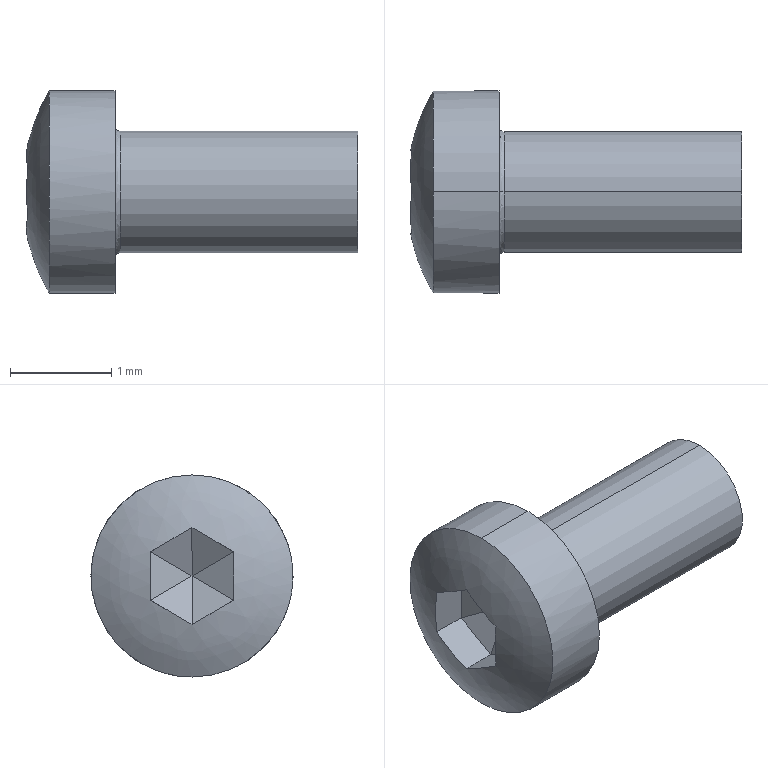Part | SolidWorks | features BaseBody 1, ICE 1, Scale 1 | 1 solid | 21 faces | box 3.277 x 2 x 2 mm | volume 4.924 mm3 | plane 14 | cylinder 4 | spline 3 | commonest cylinder face diameters 1.2 x2 2 x2
STEP:
#1=CARTESIAN_POINT('',(0.92,0.,0.65));
#2=VERTEX_POINT('',#1);
#3=CARTESIAN_POINT('',(0.92,0.,-0.65));
#4=VERTEX_POINT('',#3);
#5=CARTESIAN_POINT('',(0.92,0.,0.65));
#6=CARTESIAN_POINT('',(0.92,0.04131,0.65));
#7=CARTESIAN_POINT('',(0.92,0.1022,0.6443));
#8=CARTESIAN_POINT('',(0.92,0.1615,0.63));
#9=CARTESIAN_POINT('',(0.92,0.2006,0.6186));
#10=CARTESIAN_POINT('',(0.92,0.2184,0.6126));
#11=CARTESIAN_POINT('',(0.92,0.3226,0.5714));
#12=CARTESIAN_POINT('',(0.92,0.3962,0.523));
#13=CARTESIAN_POINT('',(0.92,0.4913,0.4279));
#14=CARTESIAN_POINT('',(0.92,0.5332,0.3766));
#15=CARTESIAN_POINT('',(0.92,0.5665,0.3196));
#16=CARTESIAN_POINT('',(0.92,0.5869,0.2804));
#17=CARTESIAN_POINT('',(0.92,0.5968,0.2585));
#18=CARTESIAN_POINT('',(0.92,0.6348,0.1625));
#19=CARTESIAN_POINT('',(0.92,0.65,0.08259));
#20=CARTESIAN_POINT('',(0.92,0.65,-0.04129));
#21=CARTESIAN_POINT('',(0.92,0.6443,-0.1022));
#22=CARTESIAN_POINT('',(0.92,0.63,-0.1615));
#23=CARTESIAN_POINT('',(0.92,0.6186,-0.2006));
#24=CARTESIAN_POINT('',(0.92,0.6126,-0.2184));
#25=CARTESIAN_POINT('',(0.92,0.5714,-0.3226));
#26=CARTESIAN_POINT('',(0.92,0.523,-0.3962));
#27=CARTESIAN_POINT('',(0.92,0.4279,-0.4913));
#28=CARTESIAN_POINT('',(0.92,0.3766,-0.5332));
#29=CARTESIAN_POINT('',(0.92,0.3196,-0.5665));
#30=CARTESIAN_POINT('',(0.92,0.2804,-0.5869));
#31=CARTESIAN_POINT('',(0.92,0.2585,-0.5968));
#32=CARTESIAN_POINT('',(0.92,0.1624,-0.6348));
#33=CARTESIAN_POINT('',(0.92,0.08269,-0.65));
#34=CARTESIAN_POINT('',(0.92,0.,-0.65));
#35=B_SPLINE_CURVE_WITH_KNOTS('',3,(#5,#6,#7,#8,#9,#10,#11,#12,#13,#14,#15,#16,#17,#18,#19,#20,#21,#22,#23,#24,#25,#26,#27,#28,#29,#30,#31,#32,#33,#34),.UNSPECIFIED.,.F.,.F.,(4,1,2,2,2,1,2,2,2,1,2,2,2,1,2,2,4),(0.,0.0625,0.09375,0.125,0.25,0.3125,0.3438,0.375,0.5,0.5625,0.5938,0.625,0.75,0.8125,0.8438,0.875,1.),.UNSPECIFIED.);
#36=EDGE_CURVE('',#2,#4,#35,.T.);
#37=ORIENTED_EDGE('',*,*,#36,.F.);
#38=CARTESIAN_POINT('',(0.97,0.,0.6));
#39=VERTEX_POINT('',#38);
#40=CARTESIAN_POINT('',(0.97,0.,0.65));
#41=DIRECTION('',(0.,-1.,0.));
#42=DIRECTION('',(0.,0.,1.));
#43=AXIS2_PLACEMENT_3D('',#40,#41,#42);
#44=CIRCLE('',#43,0.05);
#45=EDGE_CURVE('',#2,#39,#44,.T.);
#46=ORIENTED_EDGE('',*,*,#45,.T.);
#47=CARTESIAN_POINT('',(0.97,0.,-0.6));
#48=VERTEX_POINT('',#47);
#49=CARTESIAN_POINT('',(0.97,0.,0.));
#50=DIRECTION('',(1.,0.,0.));
#51=DIRECTION('',(0.,0.,1.));
#52=AXIS2_PLACEMENT_3D('',#49,#50,#51);
#53=CIRCLE('',#52,0.6);
#54=EDGE_CURVE('',#48,#39,#53,.T.);
#55=ORIENTED_EDGE('',*,*,#54,.F.);
#56=CARTESIAN_POINT('',(0.97,0.,-0.65));
#57=DIRECTION('',(0.,1.,0.));
#58=DIRECTION('',(0.,0.,-1.));
#59=AXIS2_PLACEMENT_3D('',#56,#57,#58);
#60=CIRCLE('',#59,0.05);
#61=EDGE_CURVE('',#4,#48,#60,.T.);
#62=ORIENTED_EDGE('',*,*,#61,.F.);
#63=EDGE_LOOP('',(#37,#46,#55,#62));
#64=FACE_OUTER_BOUND('',#63,.T.);
#65=CARTESIAN_POINT('',(0.92,0.,-0.65));
#66=CARTESIAN_POINT('',(0.92,1.3,-0.65));
#67=CARTESIAN_POINT('',(0.92,1.3,0.65));
#68=CARTESIAN_POINT('',(0.92,0.,0.65));
#69=CARTESIAN_POINT('',(0.92,0.,-0.6207));
#70=CARTESIAN_POINT('',(0.92,1.241,-0.6207));
#71=CARTESIAN_POINT('',(0.92,1.241,0.6207));
#72=CARTESIAN_POINT('',(0.92,0.,0.6207));
#73=CARTESIAN_POINT('',(0.9407,0.,-0.6));
#74=CARTESIAN_POINT('',(0.9407,1.2,-0.6));
#75=CARTESIAN_POINT('',(0.9407,1.2,0.6));
#76=CARTESIAN_POINT('',(0.9407,0.,0.6));
#77=CARTESIAN_POINT('',(0.97,0.,-0.6));
#78=CARTESIAN_POINT('',(0.97,1.2,-0.6));
#79=CARTESIAN_POINT('',(0.97,1.2,0.6));
#80=CARTESIAN_POINT('',(0.97,0.,0.6));
#81=(BOUNDED_SURFACE()B_SPLINE_SURFACE(3,3,((#65,#66,#67,#68),(#69,#70,#71,#72),(#73,#74,#75,#76),(#77,#78,#79,#80)),.UNSPECIFIED.,.F.,.F.,.T.)B_SPLINE_SURFACE_WITH_KNOTS((4,4),(4,4),(0.,1.),(0.,1.),.UNSPECIFIED.)GEOMETRIC_REPRESENTATION_ITEM()RATIONAL_B_SPLINE_SURFACE(((1.,0.3333,0.3333,1.),(0.8047,0.2682,0.2682,0.8047),(0.8047,0.2682,0.2682,0.8047),(1.,0.3333,0.3333,1.)))REPRESENTATION_ITEM('')SURFACE());
#82=ADVANCED_FACE('',(#64),#81,.F.);
#83=CARTESIAN_POINT('',(0.2679,0.,1.));
#84=VERTEX_POINT('',#83);
#85=CARTESIAN_POINT('',(0.2679,0.,-1.));
#86=VERTEX_POINT('',#85);
#87=CARTESIAN_POINT('',(0.2679,0.,1.));
#88=CARTESIAN_POINT('',(0.2679,0.1305,1.));
#89=CARTESIAN_POINT('',(0.2679,0.262,0.9738));
#90=CARTESIAN_POINT('',(0.2679,0.5027,0.8742));
#91=CARTESIAN_POINT('',(0.2679,0.6143,0.7997));
#92=CARTESIAN_POINT('',(0.2679,0.7989,0.6155));
#93=CARTESIAN_POINT('',(0.2679,0.8733,0.5044));
#94=CARTESIAN_POINT('',(0.2679,0.9737,0.2626));
#95=CARTESIAN_POINT('',(0.2679,0.9999,0.1327));
#96=CARTESIAN_POINT('',(0.2679,1.,-0.131));
#97=CARTESIAN_POINT('',(0.2679,0.9743,-0.2608));
#98=CARTESIAN_POINT('',(0.2679,0.8739,-0.5034));
#99=CARTESIAN_POINT('',(0.2679,0.7999,-0.6142));
#100=CARTESIAN_POINT('',(0.2679,0.5231,-0.8914));
#101=CARTESIAN_POINT('',(0.2679,0.2642,-1.));
#102=CARTESIAN_POINT('',(0.2679,0.,-1.));
#103=B_SPLINE_CURVE_WITH_KNOTS('',3,(#87,#88,#89,#90,#91,#92,#93,#94,#95,#96,#97,#98,#99,#100,#101,#102),.UNSPECIFIED.,.F.,.F.,(4,2,2,2,2,2,2,4),(0.003126,0.003517,0.003908,0.004299,0.004689,0.00508,0.005471,0.006252),.UNSPECIFIED.);
#104=EDGE_CURVE('',#84,#86,#103,.T.);
#105=ORIENTED_EDGE('',*,*,#104,.F.);
#106=CARTESIAN_POINT('',(0.92,0.,1.));
#107=VERTEX_POINT('',#106);
#108=CARTESIAN_POINT('',(-0.01516,0.,1.));
#109=DIRECTION('',(1.,0.,0.));
#110=VECTOR('',#109,1000.);
#111=LINE('',#108,#110);
#112=EDGE_CURVE('',#84,#107,#111,.T.);
#113=ORIENTED_EDGE('',*,*,#112,.T.);
#114=CARTESIAN_POINT('',(0.92,0.,-1.));
#115=VERTEX_POINT('',#114);
#116=CARTESIAN_POINT('',(0.92,0.,0.));
#117=DIRECTION('',(1.,0.,0.));
#118=DIRECTION('',(0.,0.,-1.));
#119=AXIS2_PLACEMENT_3D('',#116,#117,#118);
#120=CIRCLE('',#119,1.);
#121=EDGE_CURVE('',#115,#107,#120,.T.);
#122=ORIENTED_EDGE('',*,*,#121,.F.);
#123=CARTESIAN_POINT('',(-0.01516,0.,-1.));
#124=DIRECTION('',(1.,0.,0.));
#125=VECTOR('',#124,1000.);
#126=LINE('',#123,#125);
#127=EDGE_CURVE('',#86,#115,#126,.T.);
#128=ORIENTED_EDGE('',*,*,#127,.F.);
#129=EDGE_LOOP('',(#105,#113,#122,#128));
#130=FACE_OUTER_BOUND('',#129,.T.);
#131=CARTESIAN_POINT('',(-0.01516,0.,0.));
#132=DIRECTION('',(1.,0.,0.));
#133=DIRECTION('',(0.,0.,-1.));
#134=AXIS2_PLACEMENT_3D('',#131,#132,#133);
#135=CYLINDRICAL_SURFACE('',#134,1.);
#136=ADVANCED_FACE('',(#130),#135,.T.);
#137=CARTESIAN_POINT('',(3.32,0.,0.6));
#138=VERTEX_POINT('',#137);
#139=CARTESIAN_POINT('',(3.32,0.,-0.6));
#140=VERTEX_POINT('',#139);
#141=CARTESIAN_POINT('',(3.32,0.,0.));
#142=DIRECTION('',(-1.,0.,0.));
#143=DIRECTION('',(0.,0.,1.));
#144=AXIS2_PLACEMENT_3D('',#141,#142,#143);
#145=CIRCLE('',#144,0.6);
#146=EDGE_CURVE('',#138,#140,#145,.T.);
#147=ORIENTED_EDGE('',*,*,#146,.T.);
#148=CARTESIAN_POINT('',(3.32,0.,-0.6));
#149=DIRECTION('',(-1.,0.,0.));
#150=VECTOR('',#149,1000.);
#151=LINE('',#148,#150);
#152=EDGE_CURVE('',#140,#48,#151,.T.);
#153=ORIENTED_EDGE('',*,*,#152,.T.);
#154=ORIENTED_EDGE('',*,*,#54,.T.);
#155=CARTESIAN_POINT('',(3.32,0.,0.6));
#156=DIRECTION('',(-1.,0.,0.));
#157=VECTOR('',#156,1000.);
#158=LINE('',#155,#157);
#159=EDGE_CURVE('',#138,#39,#158,.T.);
#160=ORIENTED_EDGE('',*,*,#159,.F.);
#161=EDGE_LOOP('',(#147,#153,#154,#160));
#162=FACE_OUTER_BOUND('',#161,.T.);
#163=CARTESIAN_POINT('',(3.32,0.,0.));
#164=DIRECTION('',(-1.,0.,0.));
#165=DIRECTION('',(0.,0.,1.));
#166=AXIS2_PLACEMENT_3D('',#163,#164,#165);
#167=CYLINDRICAL_SURFACE('',#166,0.6);
#168=ADVANCED_FACE('',(#162),#167,.T.);
#169=CARTESIAN_POINT('',(0.92,0.,-0.65));
#170=CARTESIAN_POINT('',(0.92,-0.04131,-0.65));
#171=CARTESIAN_POINT('',(0.92,-0.1022,-0.6443));
#172=CARTESIAN_POINT('',(0.92,-0.1615,-0.63));
#173=CARTESIAN_POINT('',(0.92,-0.2006,-0.6186));
#174=CARTESIAN_POINT('',(0.92,-0.2184,-0.6126));
#175=CARTESIAN_POINT('',(0.92,-0.3226,-0.5714));
#176=CARTESIAN_POINT('',(0.92,-0.3962,-0.523));
#177=CARTESIAN_POINT('',(0.92,-0.4913,-0.4279));
#178=CARTESIAN_POINT('',(0.92,-0.5332,-0.3766));
#179=CARTESIAN_POINT('',(0.92,-0.5665,-0.3196));
#180=CARTESIAN_POINT('',(0.92,-0.5869,-0.2804));
#181=CARTESIAN_POINT('',(0.92,-0.5968,-0.2585));
#182=CARTESIAN_POINT('',(0.92,-0.6348,-0.1625));
#183=CARTESIAN_POINT('',(0.92,-0.65,-0.08259));
#184=CARTESIAN_POINT('',(0.92,-0.65,0.04129));
#185=CARTESIAN_POINT('',(0.92,-0.6443,0.1022));
#186=CARTESIAN_POINT('',(0.92,-0.63,0.1615));
#187=CARTESIAN_POINT('',(0.92,-0.6186,0.2006));
#188=CARTESIAN_POINT('',(0.92,-0.6126,0.2184));
#189=CARTESIAN_POINT('',(0.92,-0.5714,0.3226));
#190=CARTESIAN_POINT('',(0.92,-0.523,0.3962));
#191=CARTESIAN_POINT('',(0.92,-0.4279,0.4913));
#192=CARTESIAN_POINT('',(0.92,-0.3766,0.5332));
#193=CARTESIAN_POINT('',(0.92,-0.3196,0.5665));
#194=CARTESIAN_POINT('',(0.92,-0.2804,0.5869));
#195=CARTESIAN_POINT('',(0.92,-0.2585,0.5968));
#196=CARTESIAN_POINT('',(0.92,-0.1624,0.6348));
#197=CARTESIAN_POINT('',(0.92,-0.08269,0.65));
#198=CARTESIAN_POINT('',(0.92,0.,0.65));
#199=B_SPLINE_CURVE_WITH_KNOTS('',3,(#169,#170,#171,#172,#173,#174,#175,#176,#177,#178,#179,#180,#181,#182,#183,#184,#185,#186,#187,#188,#189,#190,#191,#192,#193,#194,#195,#196,#197,#198),.UNSPECIFIED.,.F.,.F.,(4,1,2,2,2,1,2,2,2,1,2,2,2,1,2,2,4),(0.,0.0625,0.09375,0.125,0.25,0.3125,0.3438,0.375,0.5,0.5625,0.5938,0.625,0.75,0.8125,0.8438,0.875,1.),.UNSPECIFIED.);
#200=EDGE_CURVE('',#4,#2,#199,.T.);
#201=ORIENTED_EDGE('',*,*,#200,.T.);
#202=ORIENTED_EDGE('',*,*,#36,.T.);
#203=EDGE_LOOP('',(#201,#202));
#204=FACE_BOUND('',#203,.T.);
#205=ORIENTED_EDGE('',*,*,#121,.T.);
#206=CARTESIAN_POINT('',(0.92,0.,0.));
#207=DIRECTION('',(1.,0.,0.));
#208=DIRECTION('',(0.,0.,-1.));
#209=AXIS2_PLACEMENT_3D('',#206,#207,#208);
#210=CIRCLE('',#209,1.);
#211=EDGE_CURVE('',#107,#115,#210,.T.);
#212=ORIENTED_EDGE('',*,*,#211,.T.);
#213=EDGE_LOOP('',(#205,#212));
#214=FACE_OUTER_BOUND('',#213,.T.);
#215=CARTESIAN_POINT('',(0.92,0.,0.));
#216=DIRECTION('',(1.,0.,0.));
#217=DIRECTION('',(0.,0.,-1.));
#218=AXIS2_PLACEMENT_3D('',#215,#216,#217);
#219=PLANE('',#218);
#220=ADVANCED_FACE('',(#204,#214),#219,.T.);
#221=ORIENTED_EDGE('',*,*,#152,.F.);
#222=CARTESIAN_POINT('',(3.32,0.,0.));
#223=DIRECTION('',(-1.,0.,0.));
#224=DIRECTION('',(0.,0.,1.));
#225=AXIS2_PLACEMENT_3D('',#222,#223,#224);
#226=CIRCLE('',#225,0.6);
#227=EDGE_CURVE('',#140,#138,#226,.T.);
#228=ORIENTED_EDGE('',*,*,#227,.T.);
#229=ORIENTED_EDGE('',*,*,#159,.T.);
#230=CARTESIAN_POINT('',(0.97,0.,0.));
#231=DIRECTION('',(1.,0.,0.));
#232=DIRECTION('',(0.,0.,1.));
#233=AXIS2_PLACEMENT_3D('',#230,#231,#232);
#234=CIRCLE('',#233,0.6);
#235=EDGE_CURVE('',#39,#48,#234,.T.);
#236=ORIENTED_EDGE('',*,*,#235,.T.);
#237=EDGE_LOOP('',(#221,#228,#229,#236));
#238=FACE_OUTER_BOUND('',#237,.T.);
#239=CARTESIAN_POINT('',(3.32,0.,0.));
#240=DIRECTION('',(-1.,0.,0.));
#241=DIRECTION('',(0.,0.,1.));
#242=AXIS2_PLACEMENT_3D('',#239,#240,#241);
#243=CYLINDRICAL_SURFACE('',#242,0.6);
#244=ADVANCED_FACE('',(#238),#243,.T.);
#245=ORIENTED_EDGE('',*,*,#45,.F.);
#246=ORIENTED_EDGE('',*,*,#200,.F.);
#247=ORIENTED_EDGE('',*,*,#61,.T.);
#248=ORIENTED_EDGE('',*,*,#235,.F.);
#249=EDGE_LOOP('',(#245,#246,#247,#248));
#250=FACE_OUTER_BOUND('',#249,.T.);
#251=CARTESIAN_POINT('',(0.92,0.,0.65));
#252=CARTESIAN_POINT('',(0.92,-1.3,0.65));
#253=CARTESIAN_POINT('',(0.92,-1.3,-0.65));
#254=CARTESIAN_POINT('',(0.92,0.,-0.65));
#255=CARTESIAN_POINT('',(0.92,0.,0.6207));
#256=CARTESIAN_POINT('',(0.92,-1.241,0.6207));
#257=CARTESIAN_POINT('',(0.92,-1.241,-0.6207));
#258=CARTESIAN_POINT('',(0.92,0.,-0.6207));
#259=CARTESIAN_POINT('',(0.9407,0.,0.6));
#260=CARTESIAN_POINT('',(0.9407,-1.2,0.6));
#261=CARTESIAN_POINT('',(0.9407,-1.2,-0.6));
#262=CARTESIAN_POINT('',(0.9407,0.,-0.6));
#263=CARTESIAN_POINT('',(0.97,0.,0.6));
#264=CARTESIAN_POINT('',(0.97,-1.2,0.6));
#265=CARTESIAN_POINT('',(0.97,-1.2,-0.6));
#266=CARTESIAN_POINT('',(0.97,0.,-0.6));
#267=(BOUNDED_SURFACE()B_SPLINE_SURFACE(3,3,((#251,#252,#253,#254),(#255,#256,#257,#258),(#259,#260,#261,#262),(#263,#264,#265,#266)),.UNSPECIFIED.,.F.,.F.,.F.)B_SPLINE_SURFACE_WITH_KNOTS((4,4),(4,4),(0.,1.),(0.,1.),.UNSPECIFIED.)GEOMETRIC_REPRESENTATION_ITEM()RATIONAL_B_SPLINE_SURFACE(((1.,0.3333,0.3333,1.),(0.8047,0.2682,0.2682,0.8047),(0.8047,0.2682,0.2682,0.8047),(1.,0.3333,0.3333,1.)))REPRESENTATION_ITEM('')SURFACE());
#268=ADVANCED_FACE('',(#250),#267,.F.);
#269=ORIENTED_EDGE('',*,*,#146,.F.);
#270=ORIENTED_EDGE('',*,*,#227,.F.);
#271=EDGE_LOOP('',(#269,#270));
#272=FACE_OUTER_BOUND('',#271,.T.);
#273=CARTESIAN_POINT('',(3.32,0.,0.));
#274=DIRECTION('',(1.,0.,0.));
#275=DIRECTION('',(0.,0.,-1.));
#276=AXIS2_PLACEMENT_3D('',#273,#274,#275);
#277=PLANE('',#276);
#278=ADVANCED_FACE('',(#272),#277,.T.);
#279=ORIENTED_EDGE('',*,*,#112,.F.);
#280=CARTESIAN_POINT('',(0.2679,0.,-1.));
#281=CARTESIAN_POINT('',(0.2679,-0.1321,-1.));
#282=CARTESIAN_POINT('',(0.2679,-0.2618,-0.974));
#283=CARTESIAN_POINT('',(0.2679,-0.504,-0.8736));
#284=CARTESIAN_POINT('',(0.2679,-0.615,-0.7993));
#285=CARTESIAN_POINT('',(0.2679,-0.7995,-0.6147));
#286=CARTESIAN_POINT('',(0.2679,-0.874,-0.5031));
#287=CARTESIAN_POINT('',(0.2679,-0.9737,-0.2624));
#288=CARTESIAN_POINT('',(0.2679,-1.,-0.1308));
#289=CARTESIAN_POINT('',(0.2679,-1.,0.1301));
#290=CARTESIAN_POINT('',(0.2679,-0.9741,0.2612));
#291=CARTESIAN_POINT('',(0.2679,-0.874,0.5033));
#292=CARTESIAN_POINT('',(0.2679,-0.8006,0.6136));
#293=CARTESIAN_POINT('',(0.2679,-0.614,0.8003));
#294=CARTESIAN_POINT('',(0.2679,-0.5038,0.8737));
#295=CARTESIAN_POINT('',(0.2679,-0.2614,0.9741));
#296=CARTESIAN_POINT('',(0.2679,-0.1305,1.));
#297=CARTESIAN_POINT('',(0.2679,0.,1.));
#298=B_SPLINE_CURVE_WITH_KNOTS('',3,(#280,#281,#282,#283,#284,#285,#286,#287,#288,#289,#290,#291,#292,#293,#294,#295,#296,#297),.UNSPECIFIED.,.F.,.F.,(4,2,2,2,2,2,2,2,4),(0.,0.0003908,0.0007816,0.001172,0.001563,0.001954,0.002345,0.002736,0.003126),.UNSPECIFIED.);
#299=EDGE_CURVE('',#86,#84,#298,.T.);
#300=ORIENTED_EDGE('',*,*,#299,.F.);
#301=ORIENTED_EDGE('',*,*,#127,.T.);
#302=ORIENTED_EDGE('',*,*,#211,.F.);
#303=EDGE_LOOP('',(#279,#300,#301,#302));
#304=FACE_OUTER_BOUND('',#303,.T.);
#305=CARTESIAN_POINT('',(-0.01516,0.,0.));
#306=DIRECTION('',(1.,0.,0.));
#307=DIRECTION('',(0.,0.,-1.));
#308=AXIS2_PLACEMENT_3D('',#305,#306,#307);
#309=CYLINDRICAL_SURFACE('',#308,1.);
#310=ADVANCED_FACE('',(#304),#309,.T.);
#311=CARTESIAN_POINT('',(0.6396,0.,0.));
#312=VERTEX_POINT('',#311);
#313=CARTESIAN_POINT('',(0.4,-0.415,-0.2396));
#314=VERTEX_POINT('',#313);
#315=CARTESIAN_POINT('',(0.6396,0.,0.));
#316=DIRECTION('',(-0.4472,-0.7746,-0.4472));
#317=VECTOR('',#316,1000.);
#318=LINE('',#315,#317);
#319=EDGE_CURVE('',#312,#314,#318,.T.);
#320=ORIENTED_EDGE('',*,*,#319,.F.);
#321=CARTESIAN_POINT('',(0.4,0.,-0.4792));
#322=VERTEX_POINT('',#321);
#323=CARTESIAN_POINT('',(0.4,0.,-0.4792));
#324=DIRECTION('',(-0.4472,0.,-0.8944));
#325=VECTOR('',#324,1000.);
#326=LINE('',#323,#325);
#327=EDGE_CURVE('',#312,#322,#326,.T.);
#328=ORIENTED_EDGE('',*,*,#327,.T.);
#329=CARTESIAN_POINT('',(0.4,-0.415,-0.2396));
#330=DIRECTION('',(0.,0.866,-0.5));
#331=VECTOR('',#330,1000.);
#332=LINE('',#329,#331);
#333=EDGE_CURVE('',#314,#322,#332,.T.);
#334=ORIENTED_EDGE('',*,*,#333,.F.);
#335=EDGE_LOOP('',(#320,#328,#334));
#336=FACE_OUTER_BOUND('',#335,.T.);
#337=CARTESIAN_POINT('',(0.4,-0.415,-0.2396));
#338=DIRECTION('',(0.866,-0.25,-0.433));
#339=DIRECTION('',(-0.4472,0.,-0.8944));
#340=AXIS2_PLACEMENT_3D('',#337,#338,#339);
#341=PLANE('',#340);
#342=ADVANCED_FACE('',(#336),#341,.F.);
#343=CARTESIAN_POINT('',(0.4,-0.415,0.2396));
#344=VERTEX_POINT('',#343);
#345=CARTESIAN_POINT('',(0.4,-0.415,0.2396));
#346=DIRECTION('',(0.4472,0.7746,-0.4472));
#347=VECTOR('',#346,1000.);
#348=LINE('',#345,#347);
#349=EDGE_CURVE('',#344,#312,#348,.T.);
#350=ORIENTED_EDGE('',*,*,#349,.T.);
#351=ORIENTED_EDGE('',*,*,#319,.T.);
#352=CARTESIAN_POINT('',(0.4,-0.415,0.2396));
#353=DIRECTION('',(0.,0.,-1.));
#354=VECTOR('',#353,1000.);
#355=LINE('',#352,#354);
#356=EDGE_CURVE('',#344,#314,#355,.T.);
#357=ORIENTED_EDGE('',*,*,#356,.F.);
#358=EDGE_LOOP('',(#350,#351,#357));
#359=FACE_OUTER_BOUND('',#358,.T.);
#360=CARTESIAN_POINT('',(0.4,-0.415,0.2396));
#361=DIRECTION('',(0.866,-0.5,0.));
#362=DIRECTION('',(0.5,0.866,0.));
#363=AXIS2_PLACEMENT_3D('',#360,#361,#362);
#364=PLANE('',#363);
#365=ADVANCED_FACE('',(#359),#364,.F.);
#366=CARTESIAN_POINT('',(0.4,0.,0.4792));
#367=VERTEX_POINT('',#366);
#368=CARTESIAN_POINT('',(0.4,0.,0.4792));
#369=DIRECTION('',(-0.4472,0.,0.8944));
#370=VECTOR('',#369,1000.);
#371=LINE('',#368,#370);
#372=EDGE_CURVE('',#312,#367,#371,.T.);
#373=ORIENTED_EDGE('',*,*,#372,.F.);
#374=ORIENTED_EDGE('',*,*,#349,.F.);
#375=CARTESIAN_POINT('',(0.4,0.,0.4792));
#376=DIRECTION('',(0.,-0.866,-0.5));
#377=VECTOR('',#376,1000.);
#378=LINE('',#375,#377);
#379=EDGE_CURVE('',#367,#344,#378,.T.);
#380=ORIENTED_EDGE('',*,*,#379,.F.);
#381=EDGE_LOOP('',(#373,#374,#380));
#382=FACE_OUTER_BOUND('',#381,.T.);
#383=CARTESIAN_POINT('',(0.4,0.,0.4792));
#384=DIRECTION('',(0.866,-0.25,0.433));
#385=DIRECTION('',(0.4472,0.,-0.8944));
#386=AXIS2_PLACEMENT_3D('',#383,#384,#385);
#387=PLANE('',#386);
#388=ADVANCED_FACE('',(#382),#387,.F.);
#389=CARTESIAN_POINT('',(0.4,0.415,0.2396));
#390=VERTEX_POINT('',#389);
#391=CARTESIAN_POINT('',(0.6396,0.,0.));
#392=DIRECTION('',(-0.4472,0.7746,0.4472));
#393=VECTOR('',#392,1000.);
#394=LINE('',#391,#393);
#395=EDGE_CURVE('',#312,#390,#394,.T.);
#396=ORIENTED_EDGE('',*,*,#395,.F.);
#397=ORIENTED_EDGE('',*,*,#372,.T.);
#398=CARTESIAN_POINT('',(0.4,0.415,0.2396));
#399=DIRECTION('',(0.,-0.866,0.5));
#400=VECTOR('',#399,1000.);
#401=LINE('',#398,#400);
#402=EDGE_CURVE('',#390,#367,#401,.T.);
#403=ORIENTED_EDGE('',*,*,#402,.F.);
#404=EDGE_LOOP('',(#396,#397,#403));
#405=FACE_OUTER_BOUND('',#404,.T.);
#406=CARTESIAN_POINT('',(0.4,0.415,0.2396));
#407=DIRECTION('',(0.866,0.25,0.433));
#408=DIRECTION('',(0.4472,0.,-0.8944));
#409=AXIS2_PLACEMENT_3D('',#406,#407,#408);
#410=PLANE('',#409);
#411=ADVANCED_FACE('',(#405),#410,.F.);
#412=CARTESIAN_POINT('',(0.4,0.415,-0.2396));
#413=VERTEX_POINT('',#412);
#414=CARTESIAN_POINT('',(0.4,0.415,-0.2396));
#415=DIRECTION('',(0.4472,-0.7746,0.4472));
#416=VECTOR('',#415,1000.);
#417=LINE('',#414,#416);
#418=EDGE_CURVE('',#413,#312,#417,.T.);
#419=ORIENTED_EDGE('',*,*,#418,.T.);
#420=ORIENTED_EDGE('',*,*,#395,.T.);
#421=CARTESIAN_POINT('',(0.4,0.415,-0.2396));
#422=DIRECTION('',(0.,0.,1.));
#423=VECTOR('',#422,1000.);
#424=LINE('',#421,#423);
#425=EDGE_CURVE('',#413,#390,#424,.T.);
#426=ORIENTED_EDGE('',*,*,#425,.F.);
#427=EDGE_LOOP('',(#419,#420,#426));
#428=FACE_OUTER_BOUND('',#427,.T.);
#429=CARTESIAN_POINT('',(0.4,0.415,-0.2396));
#430=DIRECTION('',(0.866,0.5,0.));
#431=DIRECTION('',(-0.5,0.866,0.));
#432=AXIS2_PLACEMENT_3D('',#429,#430,#431);
#433=PLANE('',#432);
#434=ADVANCED_FACE('',(#428),#433,.F.);
#435=ORIENTED_EDGE('',*,*,#327,.F.);
#436=ORIENTED_EDGE('',*,*,#418,.F.);
#437=CARTESIAN_POINT('',(0.4,0.,-0.4792));
#438=DIRECTION('',(0.,0.866,0.5));
#439=VECTOR('',#438,1000.);
#440=LINE('',#437,#439);
#441=EDGE_CURVE('',#322,#413,#440,.T.);
#442=ORIENTED_EDGE('',*,*,#441,.F.);
#443=EDGE_LOOP('',(#435,#436,#442));
#444=FACE_OUTER_BOUND('',#443,.T.);
#445=CARTESIAN_POINT('',(0.4,0.,-0.4792));
#446=DIRECTION('',(0.866,0.25,-0.433));
#447=DIRECTION('',(-0.4472,0.,-0.8944));
#448=AXIS2_PLACEMENT_3D('',#445,#446,#447);
#449=PLANE('',#448);
#450=ADVANCED_FACE('',(#444),#449,.F.);
#451=CARTESIAN_POINT('',(0.05826,0.,-0.4792));
#452=VERTEX_POINT('',#451);
#453=CARTESIAN_POINT('',(0.4,0.,-0.4792));
#454=DIRECTION('',(1.,0.,0.));
#455=VECTOR('',#454,1000.);
#456=LINE('',#453,#455);
#457=EDGE_CURVE('',#452,#322,#456,.T.);
#458=ORIENTED_EDGE('',*,*,#457,.F.);
#459=CARTESIAN_POINT('',(0.05826,-0.415,-0.2396));
#460=VERTEX_POINT('',#459);
#461=CARTESIAN_POINT('',(0.05826,-0.415,-0.2396));
#462=CARTESIAN_POINT('',(0.03855,-0.2767,-0.3195));
#463=CARTESIAN_POINT('',(0.03855,-0.1383,-0.3993));
#464=CARTESIAN_POINT('',(0.05826,0.,-0.4792));
#465=B_SPLINE_CURVE_WITH_KNOTS('',3,(#461,#462,#463,#464),.UNSPECIFIED.,.F.,.F.,(4,4),(0.,0.0004792),.UNSPECIFIED.);
#466=EDGE_CURVE('',#460,#452,#465,.T.);
#467=ORIENTED_EDGE('',*,*,#466,.F.);
#468=CARTESIAN_POINT('',(0.4,-0.415,-0.2396));
#469=DIRECTION('',(-1.,0.,0.));
#470=VECTOR('',#469,1000.);
#471=LINE('',#468,#470);
#472=EDGE_CURVE('',#314,#460,#471,.T.);
#473=ORIENTED_EDGE('',*,*,#472,.F.);
#474=ORIENTED_EDGE('',*,*,#333,.T.);
#475=EDGE_LOOP('',(#458,#467,#473,#474));
#476=FACE_OUTER_BOUND('',#475,.T.);
#477=CARTESIAN_POINT('',(0.4,-0.415,-0.2396));
#478=DIRECTION('',(0.,0.5,0.866));
#479=DIRECTION('',(0.,-0.866,0.5));
#480=AXIS2_PLACEMENT_3D('',#477,#478,#479);
#481=PLANE('',#480);
#482=ADVANCED_FACE('',(#476),#481,.T.);
#483=ORIENTED_EDGE('',*,*,#472,.T.);
#484=CARTESIAN_POINT('',(0.05826,-0.415,0.2396));
#485=VERTEX_POINT('',#484);
#486=CARTESIAN_POINT('',(2.,-0.415,0.));
#487=DIRECTION('',(0.,1.,0.));
#488=DIRECTION('',(0.,0.,-1.));
#489=AXIS2_PLACEMENT_3D('',#486,#487,#488);
#490=CIRCLE('',#489,1.956);
#491=EDGE_CURVE('',#460,#485,#490,.T.);
#492=ORIENTED_EDGE('',*,*,#491,.T.);
#493=CARTESIAN_POINT('',(0.4,-0.415,0.2396));
#494=DIRECTION('',(1.,0.,0.));
#495=VECTOR('',#494,1000.);
#496=LINE('',#493,#495);
#497=EDGE_CURVE('',#485,#344,#496,.T.);
#498=ORIENTED_EDGE('',*,*,#497,.T.);
#499=ORIENTED_EDGE('',*,*,#356,.T.);
#500=EDGE_LOOP('',(#483,#492,#498,#499));
#501=FACE_OUTER_BOUND('',#500,.T.);
#502=CARTESIAN_POINT('',(0.4,-0.415,0.2396));
#503=DIRECTION('',(0.,1.,0.));
#504=DIRECTION('',(0.,0.,1.));
#505=AXIS2_PLACEMENT_3D('',#502,#503,#504);
#506=PLANE('',#505);
#507=ADVANCED_FACE('',(#501),#506,.T.);
#508=ORIENTED_EDGE('',*,*,#497,.F.);
#509=CARTESIAN_POINT('',(0.05826,0.,0.4792));
#510=VERTEX_POINT('',#509);
#511=CARTESIAN_POINT('',(0.05826,0.,0.4792));
#512=CARTESIAN_POINT('',(0.03855,-0.1383,0.3993));
#513=CARTESIAN_POINT('',(0.03855,-0.2767,0.3195));
#514=CARTESIAN_POINT('',(0.05826,-0.415,0.2396));
#515=B_SPLINE_CURVE_WITH_KNOTS('',3,(#511,#512,#513,#514),.UNSPECIFIED.,.F.,.F.,(4,4),(0.,0.0004792),.UNSPECIFIED.);
#516=EDGE_CURVE('',#510,#485,#515,.T.);
#517=ORIENTED_EDGE('',*,*,#516,.F.);
#518=CARTESIAN_POINT('',(0.4,0.,0.4792));
#519=DIRECTION('',(1.,0.,0.));
#520=VECTOR('',#519,1000.);
#521=LINE('',#518,#520);
#522=EDGE_CURVE('',#510,#367,#521,.T.);
#523=ORIENTED_EDGE('',*,*,#522,.T.);
#524=ORIENTED_EDGE('',*,*,#379,.T.);
#525=EDGE_LOOP('',(#508,#517,#523,#524));
#526=FACE_OUTER_BOUND('',#525,.T.);
#527=CARTESIAN_POINT('',(0.4,0.,0.4792));
#528=DIRECTION('',(0.,0.5,-0.866));
#529=DIRECTION('',(0.,0.866,0.5));
#530=AXIS2_PLACEMENT_3D('',#527,#528,#529);
#531=PLANE('',#530);
#532=ADVANCED_FACE('',(#526),#531,.T.);
#533=ORIENTED_EDGE('',*,*,#522,.F.);
#534=CARTESIAN_POINT('',(0.05826,0.415,0.2396));
#535=VERTEX_POINT('',#534);
#536=CARTESIAN_POINT('',(0.05826,0.415,0.2396));
#537=CARTESIAN_POINT('',(0.03855,0.2767,0.3195));
#538=CARTESIAN_POINT('',(0.03855,0.1383,0.3993));
#539=CARTESIAN_POINT('',(0.05826,0.,0.4792));
#540=B_SPLINE_CURVE_WITH_KNOTS('',3,(#536,#537,#538,#539),.UNSPECIFIED.,.F.,.F.,(4,4),(0.,0.0004792),.UNSPECIFIED.);
#541=EDGE_CURVE('',#535,#510,#540,.T.);
#542=ORIENTED_EDGE('',*,*,#541,.F.);
#543=CARTESIAN_POINT('',(0.4,0.415,0.2396));
#544=DIRECTION('',(-1.,0.,0.));
#545=VECTOR('',#544,1000.);
#546=LINE('',#543,#545);
#547=EDGE_CURVE('',#390,#535,#546,.T.);
#548=ORIENTED_EDGE('',*,*,#547,.F.);
#549=ORIENTED_EDGE('',*,*,#402,.T.);
#550=EDGE_LOOP('',(#533,#542,#548,#549));
#551=FACE_OUTER_BOUND('',#550,.T.);
#552=CARTESIAN_POINT('',(0.4,0.415,0.2396));
#553=DIRECTION('',(0.,-0.5,-0.866));
#554=DIRECTION('',(0.,0.866,-0.5));
#555=AXIS2_PLACEMENT_3D('',#552,#553,#554);
#556=PLANE('',#555);
#557=ADVANCED_FACE('',(#551),#556,.T.);
#558=ORIENTED_EDGE('',*,*,#547,.T.);
#559=CARTESIAN_POINT('',(0.05826,0.415,-0.2396));
#560=VERTEX_POINT('',#559);
#561=CARTESIAN_POINT('',(2.,0.415,0.));
#562=DIRECTION('',(0.,-1.,0.));
#563=DIRECTION('',(0.,0.,-1.));
#564=AXIS2_PLACEMENT_3D('',#561,#562,#563);
#565=CIRCLE('',#564,1.956);
#566=EDGE_CURVE('',#535,#560,#565,.T.);
#567=ORIENTED_EDGE('',*,*,#566,.T.);
#568=CARTESIAN_POINT('',(0.4,0.415,-0.2396));
#569=DIRECTION('',(1.,0.,0.));
#570=VECTOR('',#569,1000.);
#571=LINE('',#568,#570);
#572=EDGE_CURVE('',#560,#413,#571,.T.);
#573=ORIENTED_EDGE('',*,*,#572,.T.);
#574=ORIENTED_EDGE('',*,*,#425,.T.);
#575=EDGE_LOOP('',(#558,#567,#573,#574));
#576=FACE_OUTER_BOUND('',#575,.T.);
#577=CARTESIAN_POINT('',(0.4,0.415,-0.2396));
#578=DIRECTION('',(0.,-1.,0.));
#579=DIRECTION('',(0.,0.,-1.));
#580=AXIS2_PLACEMENT_3D('',#577,#578,#579);
#581=PLANE('',#580);
#582=ADVANCED_FACE('',(#576),#581,.T.);
#583=ORIENTED_EDGE('',*,*,#572,.F.);
#584=CARTESIAN_POINT('',(0.05826,0.,-0.4792));
#585=CARTESIAN_POINT('',(0.03855,0.1383,-0.3993));
#586=CARTESIAN_POINT('',(0.03855,0.2767,-0.3195));
#587=CARTESIAN_POINT('',(0.05826,0.415,-0.2396));
#588=B_SPLINE_CURVE_WITH_KNOTS('',3,(#584,#585,#586,#587),.UNSPECIFIED.,.F.,.F.,(4,4),(0.,0.0004792),.UNSPECIFIED.);
#589=EDGE_CURVE('',#452,#560,#588,.T.);
#590=ORIENTED_EDGE('',*,*,#589,.F.);
#591=ORIENTED_EDGE('',*,*,#457,.T.);
#592=ORIENTED_EDGE('',*,*,#441,.T.);
#593=EDGE_LOOP('',(#583,#590,#591,#592));
#594=FACE_OUTER_BOUND('',#593,.T.);
#595=CARTESIAN_POINT('',(0.4,0.,-0.4792));
#596=DIRECTION('',(0.,-0.5,0.866));
#597=DIRECTION('',(0.,-0.866,-0.5));
#598=AXIS2_PLACEMENT_3D('',#595,#596,#597);
#599=PLANE('',#598);
#600=ADVANCED_FACE('',(#594),#599,.T.);
#601=ORIENTED_EDGE('',*,*,#589,.T.);
#602=ORIENTED_EDGE('',*,*,#566,.F.);
#603=ORIENTED_EDGE('',*,*,#541,.T.);
#604=ORIENTED_EDGE('',*,*,#516,.T.);
#605=ORIENTED_EDGE('',*,*,#491,.F.);
#606=ORIENTED_EDGE('',*,*,#466,.T.);
#607=EDGE_LOOP('',(#601,#602,#603,#604,#605,#606));
#608=FACE_BOUND('',#607,.T.);
#609=ORIENTED_EDGE('',*,*,#299,.T.);
#610=ORIENTED_EDGE('',*,*,#104,.T.);
#611=EDGE_LOOP('',(#609,#610));
#612=FACE_OUTER_BOUND('',#611,.T.);
#613=CARTESIAN_POINT('',(0.5165,-1.017,0.8744));
#614=CARTESIAN_POINT('',(0.1912,-1.017,0.3227));
#615=CARTESIAN_POINT('',(0.1904,-1.017,-0.3178));
#616=CARTESIAN_POINT('',(0.5141,-1.017,-0.8704));
#617=CARTESIAN_POINT('',(0.1901,-0.3756,1.067));
#618=CARTESIAN_POINT('',(-0.2067,-0.3756,0.3937));
#619=CARTESIAN_POINT('',(-0.2078,-0.3756,-0.3877));
#620=CARTESIAN_POINT('',(0.1872,-0.3756,-1.062));
#621=CARTESIAN_POINT('',(0.1891,0.3694,1.067));
#622=CARTESIAN_POINT('',(-0.2079,0.3694,0.3939));
#623=CARTESIAN_POINT('',(-0.2089,0.3694,-0.3879));
#624=CARTESIAN_POINT('',(0.1862,0.3694,-1.062));
#625=CARTESIAN_POINT('',(0.5139,1.012,0.8759));
#626=CARTESIAN_POINT('',(0.1881,1.012,0.3232));
#627=CARTESIAN_POINT('',(0.1873,1.012,-0.3183));
#628=CARTESIAN_POINT('',(0.5115,1.012,-0.8719));
#629=(BOUNDED_SURFACE()B_SPLINE_SURFACE(3,3,((#613,#614,#615,#616),(#617,#618,#619,#620),(#621,#622,#623,#624),(#625,#626,#627,#628)),.UNSPECIFIED.,.F.,.F.,.F.)B_SPLINE_SURFACE_WITH_KNOTS((4,4),(4,4),(0.,1.),(0.,1.),.UNSPECIFIED.)GEOMETRIC_REPRESENTATION_ITEM()RATIONAL_B_SPLINE_SURFACE(((1.,0.9081,0.9081,1.),(0.9079,0.8244,0.8244,0.9079),(0.9079,0.8244,0.8244,0.9079),(1.,0.9081,0.9081,1.)))REPRESENTATION_ITEM('')SURFACE());
#630=ADVANCED_FACE('',(#608,#612),#629,.T.);
#631=CLOSED_SHELL('',(#82,#136,#168,#220,#244,#268,#278,#310,#342,#365,#388,#411,#434,#450,#482,#507,#532,#557,#582,#600,#630));
#632=MANIFOLD_SOLID_BREP('',#631);
#633=CARTESIAN_POINT('',(0.,0.,0.));
#634=DIRECTION('',(0.,0.,1.));
#635=DIRECTION('',(1.,0.,0.));
#636=AXIS2_PLACEMENT_3D('',#633,#634,#635);
#637=(LENGTH_UNIT()NAMED_UNIT(*)SI_UNIT(.MILLI.,.METRE.));
#638=UNCERTAINTY_MEASURE_WITH_UNIT(LENGTH_MEASURE(0.00001),#637,'','');
#639=(NAMED_UNIT(*)PLANE_ANGLE_UNIT()SI_UNIT($,.RADIAN.));
#640=(NAMED_UNIT(*)SI_UNIT($,.STERADIAN.)SOLID_ANGLE_UNIT());
#641=(GEOMETRIC_REPRESENTATION_CONTEXT(3)GLOBAL_UNCERTAINTY_ASSIGNED_CONTEXT((#638))GLOBAL_UNIT_ASSIGNED_CONTEXT((#637,#639,#640))REPRESENTATION_CONTEXT('',''));
#642=ADVANCED_BREP_SHAPE_REPRESENTATION('',(#632,#636),#641);